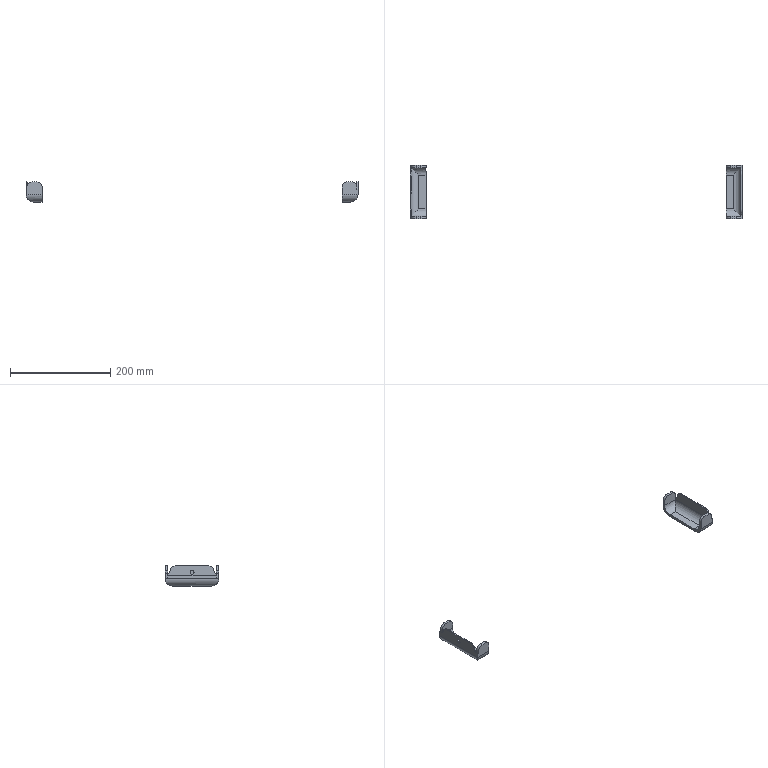Part | SolidWorks | features BaseBody 2 | 2 solids | 62 faces | box 664 x 107.82 x 40 mm | volume 66958 mm3 | plane 32 | cylinder 30 | commonest cylinder face diameters 20 x12 30 x12 10 x4 8 x2